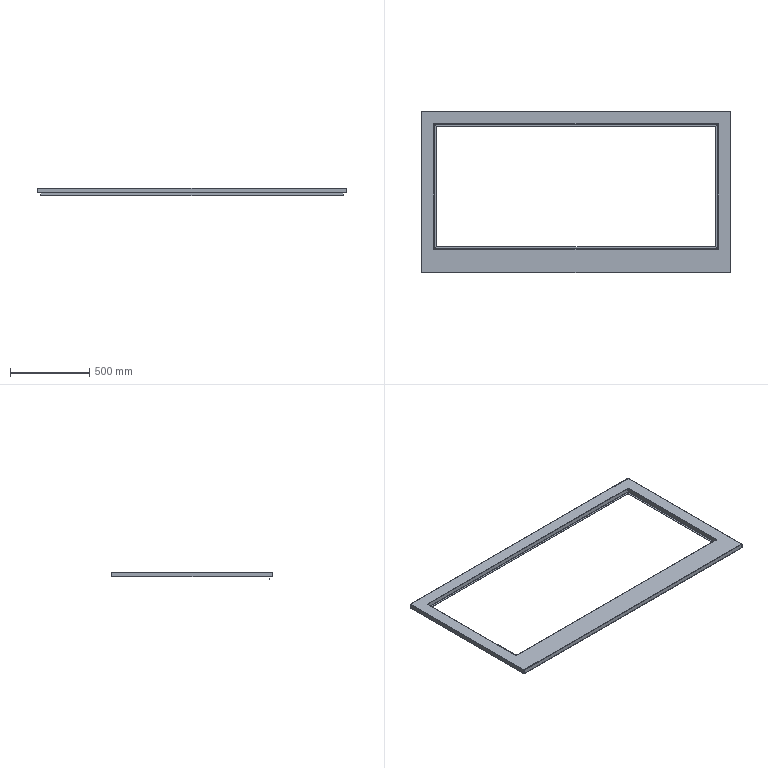Part | SolidWorks | features EdgeFlange 5, FlatPattern 1, HoleWzd 1, ICE 1, SMBaseFlange 1, SheetMetal 1 | 1 solid | 160 faces | box 1950 x 1020 x 48.5 mm | volume 1634883 mm3 | plane 86 | cylinder 42 | spline 32 | commonest cylinder face diameters 1 x17 4 x17 5 x8